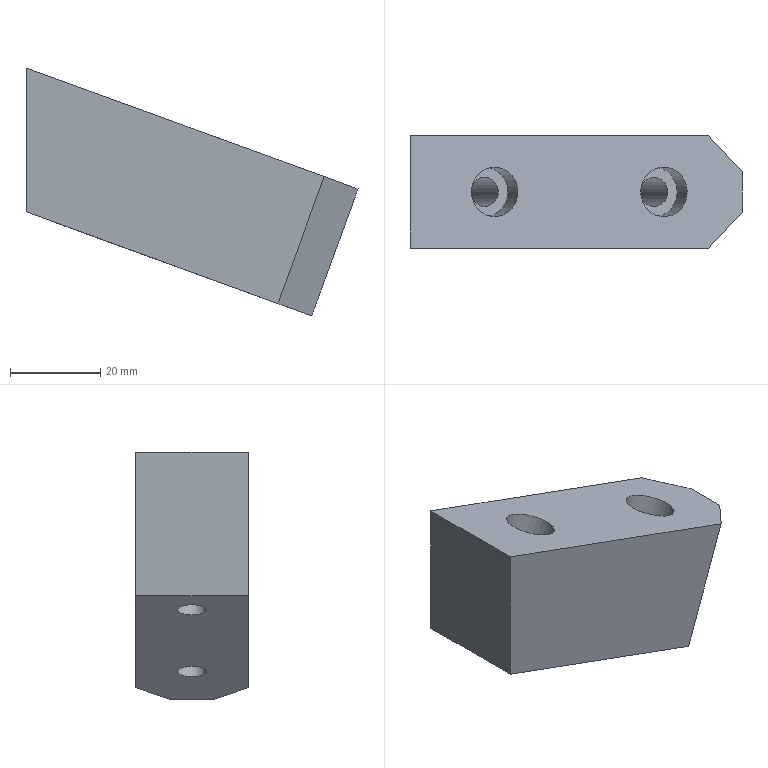Part | STEP file | P011002S002-009 | 1 solid | 14 faces | box 73.728 x 25 x 55.026 mm | volume 50035 mm3 | plane 10 | cylinder 4 | commonest cylinder face diameters 6.5 x2 11 x2
STEP:
#1=CARTESIAN_POINT('',(0.,0.,0.));
#2=DIRECTION('',(0.,0.,1.));
#3=DIRECTION('',(1.,0.,0.));
#4=AXIS2_PLACEMENT_3D('',#1,#2,#3);
#5=CARTESIAN_POINT('',(214.175,15.,-62.861));
#6=VERTEX_POINT('',#5);
#7=CARTESIAN_POINT('',(211.121,15.,-61.749));
#8=DIRECTION('',(-0.342,0.,-0.9397));
#9=DIRECTION('',(0.9397,0.,-0.342));
#10=AXIS2_PLACEMENT_3D('',#7,#8,#9);
#11=CIRCLE('',#10,3.25);
#12=CARTESIAN_POINT('',(219.07,-90.,-64.643));
#13=DIRECTION('',(0.342,0.,0.9397));
#14=DIRECTION('',(-0.9397,0.,0.342));
#15=AXIS2_PLACEMENT_3D('',#12,#13,#14);
#16=PLANE('',#15);
#17=CARTESIAN_POINT('',(5.21,-105.));
#18=CARTESIAN_POINT('',(5.21,-99.371));
#19=CARTESIAN_POINT('',(10.085,-102.185));
#20=CARTESIAN_POINT('',(14.96,-105.));
#21=CARTESIAN_POINT('',(10.085,-107.815));
#22=CARTESIAN_POINT('',(5.21,-110.629));
#23=CARTESIAN_POINT('',(5.21,-105.));
#24=(BOUNDED_CURVE()B_SPLINE_CURVE(2,(#17,#18,#19,#20,#21,#22,#23),.UNSPECIFIED.,.T.,.F.)B_SPLINE_CURVE_WITH_KNOTS((1,2,2,2,2,1),(-2.094,0.,2.094,4.189,6.283,8.378),.UNSPECIFIED.)CURVE()GEOMETRIC_REPRESENTATION_ITEM()RATIONAL_B_SPLINE_CURVE((1.,0.5,1.,0.5,1.,0.5,1.))REPRESENTATION_ITEM(''));
#25=(GEOMETRIC_REPRESENTATION_CONTEXT(2)PARAMETRIC_REPRESENTATION_CONTEXT()REPRESENTATION_CONTEXT('',''));
#26=DEFINITIONAL_REPRESENTATION('',(#24),#25);
#27=PCURVE('',#16,#26);
#28=CARTESIAN_POINT('',(221.382,15.,-33.559));
#29=DIRECTION('',(-0.342,0.,-0.9397));
#30=DIRECTION('',(0.9397,0.,-0.342));
#31=AXIS2_PLACEMENT_3D('',#28,#29,#30);
#32=CYLINDRICAL_SURFACE('',#31,3.25);
#33=CARTESIAN_POINT('',(0.,30.));
#34=DIRECTION('',(1.,0.));
#35=VECTOR('',#34,1.);
#36=LINE('',#33,#35);
#37=(GEOMETRIC_REPRESENTATION_CONTEXT(2)PARAMETRIC_REPRESENTATION_CONTEXT()REPRESENTATION_CONTEXT('',''));
#38=DEFINITIONAL_REPRESENTATION('',(#36),#37);
#39=PCURVE('',#32,#38);
#40=SURFACE_CURVE('',#11,(#27,#39),.PCURVE_S1.);
#41=EDGE_CURVE('',#6,#6,#40,.T.);
#42=ORIENTED_EDGE('',*,*,#41,.F.);
#43=EDGE_LOOP('',(#42));
#44=FACE_BOUND('',#43,.T.);
#45=CARTESIAN_POINT('',(220.95,2.5,-65.327));
#46=VERTEX_POINT('',#45);
#47=CARTESIAN_POINT('',(165.,2.5,-44.963));
#48=VERTEX_POINT('',#47);
#49=CARTESIAN_POINT('',(219.07,2.5,-64.643));
#50=DIRECTION('',(-0.9397,0.,0.342));
#51=VECTOR('',#50,1.);
#52=LINE('',#49,#51);
#53=CARTESIAN_POINT('',(0.,-92.5));
#54=DIRECTION('',(1.,0.));
#55=VECTOR('',#54,1.);
#56=LINE('',#53,#55);
#57=(GEOMETRIC_REPRESENTATION_CONTEXT(2)PARAMETRIC_REPRESENTATION_CONTEXT()REPRESENTATION_CONTEXT('',''));
#58=DEFINITIONAL_REPRESENTATION('',(#56),#57);
#59=PCURVE('',#16,#58);
#60=CARTESIAN_POINT('',(228.899,2.5,-52.257));
#61=DIRECTION('',(0.,-1.,0.));
#62=DIRECTION('',(0.342,0.,0.9397));
#63=AXIS2_PLACEMENT_3D('',#60,#61,#62);
#64=PLANE('',#63);
#65=CARTESIAN_POINT('',(-15.,5.));
#66=DIRECTION('',(0.,1.));
#67=VECTOR('',#66,1.);
#68=LINE('',#65,#67);
#69=(GEOMETRIC_REPRESENTATION_CONTEXT(2)PARAMETRIC_REPRESENTATION_CONTEXT()REPRESENTATION_CONTEXT('',''));
#70=DEFINITIONAL_REPRESENTATION('',(#68),#69);
#71=PCURVE('',#64,#70);
#72=SURFACE_CURVE('',#52,(#59,#71),.PCURVE_S1.);
#73=EDGE_CURVE('',#46,#48,#72,.T.);
#74=ORIENTED_EDGE('',*,*,#73,.T.);
#75=CARTESIAN_POINT('',(165.,27.5,-44.963));
#76=VERTEX_POINT('',#75);
#77=CARTESIAN_POINT('',(165.,-90.,-44.963));
#78=DIRECTION('',(0.,1.,0.));
#79=VECTOR('',#78,1.);
#80=LINE('',#77,#79);
#81=CARTESIAN_POINT('',(57.54,0.));
#82=DIRECTION('',(0.,-1.));
#83=VECTOR('',#82,1.);
#84=LINE('',#81,#83);
#85=(GEOMETRIC_REPRESENTATION_CONTEXT(2)PARAMETRIC_REPRESENTATION_CONTEXT()REPRESENTATION_CONTEXT('',''));
#86=DEFINITIONAL_REPRESENTATION('',(#84),#85);
#87=PCURVE('',#16,#86);
#88=CARTESIAN_POINT('',(165.,-10.,0.));
#89=DIRECTION('',(-1.,0.,0.));
#90=DIRECTION('',(0.,0.,-1.));
#91=AXIS2_PLACEMENT_3D('',#88,#89,#90);
#92=PLANE('',#91);
#93=CARTESIAN_POINT('',(44.963,80.));
#94=DIRECTION('',(0.,-1.));
#95=VECTOR('',#94,1.);
#96=LINE('',#93,#95);
#97=(GEOMETRIC_REPRESENTATION_CONTEXT(2)PARAMETRIC_REPRESENTATION_CONTEXT()REPRESENTATION_CONTEXT('',''));
#98=DEFINITIONAL_REPRESENTATION('',(#96),#97);
#99=PCURVE('',#92,#98);
#100=SURFACE_CURVE('',#80,(#87,#99),.PCURVE_S1.);
#101=EDGE_CURVE('',#48,#76,#100,.T.);
#102=ORIENTED_EDGE('',*,*,#101,.T.);
#103=CARTESIAN_POINT('',(220.95,27.5,-65.327));
#104=VERTEX_POINT('',#103);
#105=CARTESIAN_POINT('',(219.07,27.5,-64.643));
#106=DIRECTION('',(0.9397,0.,-0.342));
#107=VECTOR('',#106,1.);
#108=LINE('',#105,#107);
#109=CARTESIAN_POINT('',(0.,-117.5));
#110=DIRECTION('',(-1.,0.));
#111=VECTOR('',#110,1.);
#112=LINE('',#109,#111);
#113=(GEOMETRIC_REPRESENTATION_CONTEXT(2)PARAMETRIC_REPRESENTATION_CONTEXT()REPRESENTATION_CONTEXT('',''));
#114=DEFINITIONAL_REPRESENTATION('',(#112),#113);
#115=PCURVE('',#16,#114);
#116=CARTESIAN_POINT('',(228.899,27.5,-52.257));
#117=DIRECTION('',(0.,1.,0.));
#118=DIRECTION('',(-0.342,0.,-0.9397));
#119=AXIS2_PLACEMENT_3D('',#116,#117,#118);
#120=PLANE('',#119);
#121=CARTESIAN_POINT('',(15.,5.));
#122=DIRECTION('',(0.,-1.));
#123=VECTOR('',#122,1.);
#124=LINE('',#121,#123);
#125=(GEOMETRIC_REPRESENTATION_CONTEXT(2)PARAMETRIC_REPRESENTATION_CONTEXT()REPRESENTATION_CONTEXT('',''));
#126=DEFINITIONAL_REPRESENTATION('',(#124),#125);
#127=PCURVE('',#120,#126);
#128=SURFACE_CURVE('',#108,(#115,#127),.PCURVE_S1.);
#129=EDGE_CURVE('',#76,#104,#128,.T.);
#130=ORIENTED_EDGE('',*,*,#129,.T.);
#131=CARTESIAN_POINT('',(228.467,19.5,-68.063));
#132=VERTEX_POINT('',#131);
#133=CARTESIAN_POINT('',(228.467,19.5,-68.063));
#134=DIRECTION('',(-0.6645,0.7071,0.2418));
#135=VECTOR('',#134,1.);
#136=LINE('',#133,#135);
#137=CARTESIAN_POINT('',(-10.,-109.5));
#138=DIRECTION('',(0.7071,-0.7071));
#139=VECTOR('',#138,1.);
#140=LINE('',#137,#139);
#141=(GEOMETRIC_REPRESENTATION_CONTEXT(2)PARAMETRIC_REPRESENTATION_CONTEXT()REPRESENTATION_CONTEXT('',''));
#142=DEFINITIONAL_REPRESENTATION('',(#140),#141);
#143=PCURVE('',#16,#142);
#144=CARTESIAN_POINT('',(233.598,19.5,-53.967));
#145=DIRECTION('',(-0.6645,-0.7071,0.2418));
#146=DIRECTION('',(-0.7287,0.6848,0.));
#147=AXIS2_PLACEMENT_3D('',#144,#145,#146);
#148=PLANE('',#147);
#149=CARTESIAN_POINT('',(3.739,14.527));
#150=DIRECTION('',(0.9684,-0.2492));
#151=VECTOR('',#150,1.);
#152=LINE('',#149,#151);
#153=(GEOMETRIC_REPRESENTATION_CONTEXT(2)PARAMETRIC_REPRESENTATION_CONTEXT()REPRESENTATION_CONTEXT('',''));
#154=DEFINITIONAL_REPRESENTATION('',(#152),#153);
#155=PCURVE('',#148,#154);
#156=SURFACE_CURVE('',#136,(#143,#155),.PCURVE_S1.);
#157=EDGE_CURVE('',#132,#104,#156,.T.);
#158=ORIENTED_EDGE('',*,*,#157,.F.);
#159=CARTESIAN_POINT('',(228.467,10.5,-68.063));
#160=VERTEX_POINT('',#159);
#161=CARTESIAN_POINT('',(228.467,-90.,-68.063));
#162=DIRECTION('',(0.,-1.,0.));
#163=VECTOR('',#162,1.);
#164=LINE('',#161,#163);
#165=CARTESIAN_POINT('',(-10.,0.));
#166=DIRECTION('',(0.,1.));
#167=VECTOR('',#166,1.);
#168=LINE('',#165,#167);
#169=(GEOMETRIC_REPRESENTATION_CONTEXT(2)PARAMETRIC_REPRESENTATION_CONTEXT()REPRESENTATION_CONTEXT('',''));
#170=DEFINITIONAL_REPRESENTATION('',(#168),#169);
#171=PCURVE('',#16,#170);
#172=CARTESIAN_POINT('',(233.598,10.,-53.967));
#173=DIRECTION('',(0.9397,0.,-0.342));
#174=DIRECTION('',(0.342,0.,0.9397));
#175=AXIS2_PLACEMENT_3D('',#172,#173,#174);
#176=PLANE('',#175);
#177=CARTESIAN_POINT('',(-15.,100.));
#178=DIRECTION('',(0.,1.));
#179=VECTOR('',#178,1.);
#180=LINE('',#177,#179);
#181=(GEOMETRIC_REPRESENTATION_CONTEXT(2)PARAMETRIC_REPRESENTATION_CONTEXT()REPRESENTATION_CONTEXT('',''));
#182=DEFINITIONAL_REPRESENTATION('',(#180),#181);
#183=PCURVE('',#176,#182);
#184=SURFACE_CURVE('',#164,(#171,#183),.PCURVE_S1.);
#185=EDGE_CURVE('',#132,#160,#184,.T.);
#186=ORIENTED_EDGE('',*,*,#185,.T.);
#187=CARTESIAN_POINT('',(220.95,2.5,-65.327));
#188=DIRECTION('',(0.6645,0.7071,-0.2418));
#189=VECTOR('',#188,1.);
#190=LINE('',#187,#189);
#191=CARTESIAN_POINT('',(-2.,-92.5));
#192=DIRECTION('',(-0.7071,-0.7071));
#193=VECTOR('',#192,1.);
#194=LINE('',#191,#193);
#195=(GEOMETRIC_REPRESENTATION_CONTEXT(2)PARAMETRIC_REPRESENTATION_CONTEXT()REPRESENTATION_CONTEXT('',''));
#196=DEFINITIONAL_REPRESENTATION('',(#194),#195);
#197=PCURVE('',#16,#196);
#198=CARTESIAN_POINT('',(226.08,2.5,-51.231));
#199=DIRECTION('',(-0.6645,0.7071,0.2418));
#200=DIRECTION('',(0.7287,0.6848,0.));
#201=AXIS2_PLACEMENT_3D('',#198,#199,#200);
#202=PLANE('',#201);
#203=CARTESIAN_POINT('',(-3.739,14.527));
#204=DIRECTION('',(0.9684,0.2492));
#205=VECTOR('',#204,1.);
#206=LINE('',#203,#205);
#207=(GEOMETRIC_REPRESENTATION_CONTEXT(2)PARAMETRIC_REPRESENTATION_CONTEXT()REPRESENTATION_CONTEXT('',''));
#208=DEFINITIONAL_REPRESENTATION('',(#206),#207);
#209=PCURVE('',#202,#208);
#210=SURFACE_CURVE('',#190,(#197,#209),.PCURVE_S1.);
#211=EDGE_CURVE('',#46,#160,#210,.T.);
#212=ORIENTED_EDGE('',*,*,#211,.F.);
#213=EDGE_LOOP('',(#74,#102,#130,#158,#186,#212));
#214=FACE_BOUND('',#213,.T.);
#215=CARTESIAN_POINT('',(176.587,15.,-49.18));
#216=VERTEX_POINT('',#215);
#217=CARTESIAN_POINT('',(173.533,15.,-48.069));
#218=DIRECTION('',(-0.342,0.,-0.9397));
#219=DIRECTION('',(0.9397,0.,-0.342));
#220=AXIS2_PLACEMENT_3D('',#217,#218,#219);
#221=CIRCLE('',#220,3.25);
#222=CARTESIAN_POINT('',(45.21,-105.));
#223=CARTESIAN_POINT('',(45.21,-99.371));
#224=CARTESIAN_POINT('',(50.085,-102.185));
#225=CARTESIAN_POINT('',(54.96,-105.));
#226=CARTESIAN_POINT('',(50.085,-107.815));
#227=CARTESIAN_POINT('',(45.21,-110.629));
#228=CARTESIAN_POINT('',(45.21,-105.));
#229=(BOUNDED_CURVE()B_SPLINE_CURVE(2,(#222,#223,#224,#225,#226,#227,#228),.UNSPECIFIED.,.T.,.F.)B_SPLINE_CURVE_WITH_KNOTS((1,2,2,2,2,1),(-2.094,0.,2.094,4.189,6.283,8.378),.UNSPECIFIED.)CURVE()GEOMETRIC_REPRESENTATION_ITEM()RATIONAL_B_SPLINE_CURVE((1.,0.5,1.,0.5,1.,0.5,1.))REPRESENTATION_ITEM(''));
#230=(GEOMETRIC_REPRESENTATION_CONTEXT(2)PARAMETRIC_REPRESENTATION_CONTEXT()REPRESENTATION_CONTEXT('',''));
#231=DEFINITIONAL_REPRESENTATION('',(#229),#230);
#232=PCURVE('',#16,#231);
#233=CARTESIAN_POINT('',(183.794,15.,-19.878));
#234=DIRECTION('',(-0.342,0.,-0.9397));
#235=DIRECTION('',(0.9397,0.,-0.342));
#236=AXIS2_PLACEMENT_3D('',#233,#234,#235);
#237=CYLINDRICAL_SURFACE('',#236,3.25);
#238=CARTESIAN_POINT('',(0.,30.));
#239=DIRECTION('',(1.,0.));
#240=VECTOR('',#239,1.);
#241=LINE('',#238,#240);
#242=(GEOMETRIC_REPRESENTATION_CONTEXT(2)PARAMETRIC_REPRESENTATION_CONTEXT()REPRESENTATION_CONTEXT('',''));
#243=DEFINITIONAL_REPRESENTATION('',(#241),#242);
#244=PCURVE('',#237,#243);
#245=SURFACE_CURVE('',#221,(#232,#244),.PCURVE_S1.);
#246=EDGE_CURVE('',#216,#216,#245,.T.);
#247=ORIENTED_EDGE('',*,*,#246,.F.);
#248=EDGE_LOOP('',(#247));
#249=FACE_BOUND('',#248,.T.);
#250=ADVANCED_FACE('',(#44,#214,#249),#16,.F.);
#251=CARTESIAN_POINT('',(165.,2.5,-13.037));
#252=VERTEX_POINT('',#251);
#253=CARTESIAN_POINT('',(231.21,2.5,-37.136));
#254=VERTEX_POINT('',#253);
#255=CARTESIAN_POINT('',(234.029,2.5,-38.162));
#256=DIRECTION('',(0.9397,0.,-0.342));
#257=VECTOR('',#256,1.);
#258=LINE('',#255,#257);
#259=CARTESIAN_POINT('',(15.,0.));
#260=DIRECTION('',(0.,-1.));
#261=VECTOR('',#260,1.);
#262=LINE('',#259,#261);
#263=(GEOMETRIC_REPRESENTATION_CONTEXT(2)PARAMETRIC_REPRESENTATION_CONTEXT()REPRESENTATION_CONTEXT('',''));
#264=DEFINITIONAL_REPRESENTATION('',(#262),#263);
#265=PCURVE('',#64,#264);
#266=CARTESIAN_POINT('',(234.029,10.,-38.162));
#267=DIRECTION('',(0.342,0.,0.9397));
#268=DIRECTION('',(-0.9397,0.,0.342));
#269=AXIS2_PLACEMENT_3D('',#266,#267,#268);
#270=PLANE('',#269);
#271=CARTESIAN_POINT('',(0.,7.5));
#272=DIRECTION('',(-1.,0.));
#273=VECTOR('',#272,1.);
#274=LINE('',#271,#273);
#275=(GEOMETRIC_REPRESENTATION_CONTEXT(2)PARAMETRIC_REPRESENTATION_CONTEXT()REPRESENTATION_CONTEXT('',''));
#276=DEFINITIONAL_REPRESENTATION('',(#274),#275);
#277=PCURVE('',#270,#276);
#278=SURFACE_CURVE('',#258,(#265,#277),.PCURVE_S1.);
#279=EDGE_CURVE('',#252,#254,#278,.T.);
#280=ORIENTED_EDGE('',*,*,#279,.F.);
#281=CARTESIAN_POINT('',(165.,2.5,0.));
#282=DIRECTION('',(0.,0.,-1.));
#283=VECTOR('',#282,1.);
#284=LINE('',#281,#283);
#285=CARTESIAN_POINT('',(27.251,77.919));
#286=DIRECTION('',(-0.9397,-0.342));
#287=VECTOR('',#286,1.);
#288=LINE('',#285,#287);
#289=(GEOMETRIC_REPRESENTATION_CONTEXT(2)PARAMETRIC_REPRESENTATION_CONTEXT()REPRESENTATION_CONTEXT('',''));
#290=DEFINITIONAL_REPRESENTATION('',(#288),#289);
#291=PCURVE('',#64,#290);
#292=CARTESIAN_POINT('',(0.,-12.5));
#293=DIRECTION('',(1.,0.));
#294=VECTOR('',#293,1.);
#295=LINE('',#292,#294);
#296=(GEOMETRIC_REPRESENTATION_CONTEXT(2)PARAMETRIC_REPRESENTATION_CONTEXT()REPRESENTATION_CONTEXT('',''));
#297=DEFINITIONAL_REPRESENTATION('',(#295),#296);
#298=PCURVE('',#92,#297);
#299=SURFACE_CURVE('',#284,(#291,#298),.PCURVE_S1.);
#300=EDGE_CURVE('',#252,#48,#299,.T.);
#301=ORIENTED_EDGE('',*,*,#300,.T.);
#302=ORIENTED_EDGE('',*,*,#73,.F.);
#303=CARTESIAN_POINT('',(226.08,2.5,-51.231));
#304=DIRECTION('',(-0.342,0.,-0.9397));
#305=VECTOR('',#304,1.);
#306=LINE('',#303,#305);
#307=CARTESIAN_POINT('',(0.,3.));
#308=DIRECTION('',(-1.,0.));
#309=VECTOR('',#308,1.);
#310=LINE('',#307,#309);
#311=(GEOMETRIC_REPRESENTATION_CONTEXT(2)PARAMETRIC_REPRESENTATION_CONTEXT()REPRESENTATION_CONTEXT('',''));
#312=DEFINITIONAL_REPRESENTATION('',(#310),#311);
#313=PCURVE('',#64,#312);
#314=CARTESIAN_POINT('',(0.,0.));
#315=DIRECTION('',(-0.2492,0.9684));
#316=VECTOR('',#315,1.);
#317=LINE('',#314,#316);
#318=(GEOMETRIC_REPRESENTATION_CONTEXT(2)PARAMETRIC_REPRESENTATION_CONTEXT()REPRESENTATION_CONTEXT('',''));
#319=DEFINITIONAL_REPRESENTATION('',(#317),#318);
#320=PCURVE('',#202,#319);
#321=SURFACE_CURVE('',#306,(#313,#320),.PCURVE_S1.);
#322=EDGE_CURVE('',#254,#46,#321,.T.);
#323=ORIENTED_EDGE('',*,*,#322,.F.);
#324=EDGE_LOOP('',(#280,#301,#302,#323));
#325=FACE_BOUND('',#324,.T.);
#326=ADVANCED_FACE('',(#325),#64,.T.);
#327=ORIENTED_EDGE('',*,*,#300,.F.);
#328=CARTESIAN_POINT('',(165.,27.5,-13.037));
#329=VERTEX_POINT('',#328);
#330=CARTESIAN_POINT('',(165.,-10.,-13.037));
#331=DIRECTION('',(0.,-1.,0.));
#332=VECTOR('',#331,1.);
#333=LINE('',#330,#332);
#334=CARTESIAN_POINT('',(13.037,0.));
#335=DIRECTION('',(0.,1.));
#336=VECTOR('',#335,1.);
#337=LINE('',#334,#336);
#338=(GEOMETRIC_REPRESENTATION_CONTEXT(2)PARAMETRIC_REPRESENTATION_CONTEXT()REPRESENTATION_CONTEXT('',''));
#339=DEFINITIONAL_REPRESENTATION('',(#337),#338);
#340=PCURVE('',#92,#339);
#341=CARTESIAN_POINT('',(73.46,20.));
#342=DIRECTION('',(0.,1.));
#343=VECTOR('',#342,1.);
#344=LINE('',#341,#343);
#345=(GEOMETRIC_REPRESENTATION_CONTEXT(2)PARAMETRIC_REPRESENTATION_CONTEXT()REPRESENTATION_CONTEXT('',''));
#346=DEFINITIONAL_REPRESENTATION('',(#344),#345);
#347=PCURVE('',#270,#346);
#348=SURFACE_CURVE('',#333,(#340,#347),.PCURVE_S1.);
#349=EDGE_CURVE('',#329,#252,#348,.T.);
#350=ORIENTED_EDGE('',*,*,#349,.F.);
#351=CARTESIAN_POINT('',(165.,27.5,-52.257));
#352=DIRECTION('',(0.,0.,-1.));
#353=VECTOR('',#352,1.);
#354=LINE('',#351,#353);
#355=CARTESIAN_POINT('',(52.257,-37.5));
#356=DIRECTION('',(1.,0.));
#357=VECTOR('',#356,1.);
#358=LINE('',#355,#357);
#359=(GEOMETRIC_REPRESENTATION_CONTEXT(2)PARAMETRIC_REPRESENTATION_CONTEXT()REPRESENTATION_CONTEXT('',''));
#360=DEFINITIONAL_REPRESENTATION('',(#358),#359);
#361=PCURVE('',#92,#360);
#362=CARTESIAN_POINT('',(21.855,60.046));
#363=DIRECTION('',(0.9397,-0.342));
#364=VECTOR('',#363,1.);
#365=LINE('',#362,#364);
#366=(GEOMETRIC_REPRESENTATION_CONTEXT(2)PARAMETRIC_REPRESENTATION_CONTEXT()REPRESENTATION_CONTEXT('',''));
#367=DEFINITIONAL_REPRESENTATION('',(#365),#366);
#368=PCURVE('',#120,#367);
#369=SURFACE_CURVE('',#354,(#361,#368),.PCURVE_S1.);
#370=EDGE_CURVE('',#329,#76,#369,.T.);
#371=ORIENTED_EDGE('',*,*,#370,.T.);
#372=ORIENTED_EDGE('',*,*,#101,.F.);
#373=EDGE_LOOP('',(#327,#350,#371,#372));
#374=FACE_BOUND('',#373,.T.);
#375=ADVANCED_FACE('',(#374),#92,.T.);
#376=ORIENTED_EDGE('',*,*,#129,.F.);
#377=ORIENTED_EDGE('',*,*,#370,.F.);
#378=CARTESIAN_POINT('',(231.21,27.5,-37.136));
#379=VERTEX_POINT('',#378);
#380=CARTESIAN_POINT('',(234.029,27.5,-38.162));
#381=DIRECTION('',(-0.9397,0.,0.342));
#382=VECTOR('',#381,1.);
#383=LINE('',#380,#382);
#384=CARTESIAN_POINT('',(-15.,0.));
#385=DIRECTION('',(0.,1.));
#386=VECTOR('',#385,1.);
#387=LINE('',#384,#386);
#388=(GEOMETRIC_REPRESENTATION_CONTEXT(2)PARAMETRIC_REPRESENTATION_CONTEXT()REPRESENTATION_CONTEXT('',''));
#389=DEFINITIONAL_REPRESENTATION('',(#387),#388);
#390=PCURVE('',#120,#389);
#391=CARTESIAN_POINT('',(0.,-17.5));
#392=DIRECTION('',(1.,0.));
#393=VECTOR('',#392,1.);
#394=LINE('',#391,#393);
#395=(GEOMETRIC_REPRESENTATION_CONTEXT(2)PARAMETRIC_REPRESENTATION_CONTEXT()REPRESENTATION_CONTEXT('',''));
#396=DEFINITIONAL_REPRESENTATION('',(#394),#395);
#397=PCURVE('',#270,#396);
#398=SURFACE_CURVE('',#383,(#390,#397),.PCURVE_S1.);
#399=EDGE_CURVE('',#379,#329,#398,.T.);
#400=ORIENTED_EDGE('',*,*,#399,.F.);
#401=CARTESIAN_POINT('',(226.08,27.5,-51.231));
#402=DIRECTION('',(0.342,0.,0.9397));
#403=VECTOR('',#402,1.);
#404=LINE('',#401,#403);
#405=CARTESIAN_POINT('',(0.,3.));
#406=DIRECTION('',(-1.,0.));
#407=VECTOR('',#406,1.);
#408=LINE('',#405,#407);
#409=(GEOMETRIC_REPRESENTATION_CONTEXT(2)PARAMETRIC_REPRESENTATION_CONTEXT()REPRESENTATION_CONTEXT('',''));
#410=DEFINITIONAL_REPRESENTATION('',(#408),#409);
#411=PCURVE('',#120,#410);
#412=CARTESIAN_POINT('',(10.957,-2.82));
#413=DIRECTION('',(-0.2492,-0.9684));
#414=VECTOR('',#413,1.);
#415=LINE('',#412,#414);
#416=(GEOMETRIC_REPRESENTATION_CONTEXT(2)PARAMETRIC_REPRESENTATION_CONTEXT()REPRESENTATION_CONTEXT('',''));
#417=DEFINITIONAL_REPRESENTATION('',(#415),#416);
#418=PCURVE('',#148,#417);
#419=SURFACE_CURVE('',#404,(#411,#418),.PCURVE_S1.);
#420=EDGE_CURVE('',#104,#379,#419,.T.);
#421=ORIENTED_EDGE('',*,*,#420,.F.);
#422=EDGE_LOOP('',(#376,#377,#400,#421));
#423=FACE_BOUND('',#422,.T.);
#424=ADVANCED_FACE('',(#423),#120,.T.);
#425=CARTESIAN_POINT('',(216.213,15.,-31.677));
#426=VERTEX_POINT('',#425);
#427=CARTESIAN_POINT('',(221.382,15.,-33.559));
#428=DIRECTION('',(-0.342,0.,-0.9397));
#429=DIRECTION('',(-0.9397,0.,0.342));
#430=AXIS2_PLACEMENT_3D('',#427,#428,#429);
#431=CIRCLE('',#430,5.5);
#432=CARTESIAN_POINT('',(18.96,-5.));
#433=CARTESIAN_POINT('',(18.96,-14.526));
#434=CARTESIAN_POINT('',(10.71,-9.763));
#435=CARTESIAN_POINT('',(2.46,-5.));
#436=CARTESIAN_POINT('',(10.71,-0.2369));
#437=CARTESIAN_POINT('',(18.96,4.526));
#438=CARTESIAN_POINT('',(18.96,-5.));
#439=(BOUNDED_CURVE()B_SPLINE_CURVE(2,(#432,#433,#434,#435,#436,#437,#438),.UNSPECIFIED.,.T.,.F.)B_SPLINE_CURVE_WITH_KNOTS((1,2,2,2,2,1),(-2.094,0.,2.094,4.189,6.283,8.378),.UNSPECIFIED.)CURVE()GEOMETRIC_REPRESENTATION_ITEM()RATIONAL_B_SPLINE_CURVE((1.,0.5,1.,0.5,1.,0.5,1.))REPRESENTATION_ITEM(''));
#440=(GEOMETRIC_REPRESENTATION_CONTEXT(2)PARAMETRIC_REPRESENTATION_CONTEXT()REPRESENTATION_CONTEXT('',''));
#441=DEFINITIONAL_REPRESENTATION('',(#439),#440);
#442=PCURVE('',#270,#441);
#443=CARTESIAN_POINT('',(221.382,15.,-33.559));
#444=DIRECTION('',(-0.342,0.,-0.9397));
#445=DIRECTION('',(0.9397,0.,-0.342));
#446=AXIS2_PLACEMENT_3D('',#443,#444,#445);
#447=CYLINDRICAL_SURFACE('',#446,5.5);
#448=CARTESIAN_POINT('',(3.142,0.));
#449=DIRECTION('',(1.,0.));
#450=VECTOR('',#449,1.);
#451=LINE('',#448,#450);
#452=(GEOMETRIC_REPRESENTATION_CONTEXT(2)PARAMETRIC_REPRESENTATION_CONTEXT()REPRESENTATION_CONTEXT('',''));
#453=DEFINITIONAL_REPRESENTATION('',(#451),#452);
#454=PCURVE('',#447,#453);
#455=SURFACE_CURVE('',#431,(#442,#454),.PCURVE_S1.);
#456=EDGE_CURVE('',#426,#426,#455,.T.);
#457=ORIENTED_EDGE('',*,*,#456,.T.);
#458=EDGE_LOOP('',(#457));
#459=FACE_BOUND('',#458,.T.);
#460=CARTESIAN_POINT('',(178.626,15.,-17.997));
#461=VERTEX_POINT('',#460);
#462=CARTESIAN_POINT('',(183.794,15.,-19.878));
#463=DIRECTION('',(-0.342,0.,-0.9397));
#464=DIRECTION('',(-0.9397,0.,0.342));
#465=AXIS2_PLACEMENT_3D('',#462,#463,#464);
#466=CIRCLE('',#465,5.5);
#467=CARTESIAN_POINT('',(58.96,-5.));
#468=CARTESIAN_POINT('',(58.96,-14.526));
#469=CARTESIAN_POINT('',(50.71,-9.763));
#470=CARTESIAN_POINT('',(42.46,-5.));
#471=CARTESIAN_POINT('',(50.71,-0.2369));
#472=CARTESIAN_POINT('',(58.96,4.526));
#473=CARTESIAN_POINT('',(58.96,-5.));
#474=(BOUNDED_CURVE()B_SPLINE_CURVE(2,(#467,#468,#469,#470,#471,#472,#473),.UNSPECIFIED.,.T.,.F.)B_SPLINE_CURVE_WITH_KNOTS((1,2,2,2,2,1),(-2.094,0.,2.094,4.189,6.283,8.378),.UNSPECIFIED.)CURVE()GEOMETRIC_REPRESENTATION_ITEM()RATIONAL_B_SPLINE_CURVE((1.,0.5,1.,0.5,1.,0.5,1.))REPRESENTATION_ITEM(''));
#475=(GEOMETRIC_REPRESENTATION_CONTEXT(2)PARAMETRIC_REPRESENTATION_CONTEXT()REPRESENTATION_CONTEXT('',''));
#476=DEFINITIONAL_REPRESENTATION('',(#474),#475);
#477=PCURVE('',#270,#476);
#478=CARTESIAN_POINT('',(183.794,15.,-19.878));
#479=DIRECTION('',(-0.342,0.,-0.9397));
#480=DIRECTION('',(0.9397,0.,-0.342));
#481=AXIS2_PLACEMENT_3D('',#478,#479,#480);
#482=CYLINDRICAL_SURFACE('',#481,5.5);
#483=CARTESIAN_POINT('',(3.142,0.));
#484=DIRECTION('',(1.,0.));
#485=VECTOR('',#484,1.);
#486=LINE('',#483,#485);
#487=(GEOMETRIC_REPRESENTATION_CONTEXT(2)PARAMETRIC_REPRESENTATION_CONTEXT()REPRESENTATION_CONTEXT('',''));
#488=DEFINITIONAL_REPRESENTATION('',(#486),#487);
#489=PCURVE('',#482,#488);
#490=SURFACE_CURVE('',#466,(#477,#489),.PCURVE_S1.);
#491=EDGE_CURVE('',#461,#461,#490,.T.);
#492=ORIENTED_EDGE('',*,*,#491,.T.);
#493=EDGE_LOOP('',(#492));
#494=FACE_BOUND('',#493,.T.);
#495=CARTESIAN_POINT('',(238.728,10.5,-39.872));
#496=VERTEX_POINT('',#495);
#497=CARTESIAN_POINT('',(238.728,19.5,-39.872));
#498=VERTEX_POINT('',#497);
#499=CARTESIAN_POINT('',(238.728,10.,-39.872));
#500=DIRECTION('',(0.,1.,0.));
#501=VECTOR('',#500,1.);
#502=LINE('',#499,#501);
#503=CARTESIAN_POINT('',(-5.,0.));
#504=DIRECTION('',(0.,-1.));
#505=VECTOR('',#504,1.);
#506=LINE('',#503,#505);
#507=(GEOMETRIC_REPRESENTATION_CONTEXT(2)PARAMETRIC_REPRESENTATION_CONTEXT()REPRESENTATION_CONTEXT('',''));
#508=DEFINITIONAL_REPRESENTATION('',(#506),#507);
#509=PCURVE('',#270,#508);
#510=CARTESIAN_POINT('',(15.,0.));
#511=DIRECTION('',(0.,-1.));
#512=VECTOR('',#511,1.);
#513=LINE('',#510,#512);
#514=(GEOMETRIC_REPRESENTATION_CONTEXT(2)PARAMETRIC_REPRESENTATION_CONTEXT()REPRESENTATION_CONTEXT('',''));
#515=DEFINITIONAL_REPRESENTATION('',(#513),#514);
#516=PCURVE('',#176,#515);
#517=SURFACE_CURVE('',#502,(#509,#516),.PCURVE_S1.);
#518=EDGE_CURVE('',#496,#498,#517,.T.);
#519=ORIENTED_EDGE('',*,*,#518,.T.);
#520=CARTESIAN_POINT('',(240.842,17.25,-40.642));
#521=DIRECTION('',(0.6645,-0.7071,-0.2418));
#522=VECTOR('',#521,1.);
#523=LINE('',#520,#522);
#524=CARTESIAN_POINT('',(-7.25,-7.25));
#525=DIRECTION('',(-0.7071,0.7071));
#526=VECTOR('',#525,1.);
#527=LINE('',#524,#526);
#528=(GEOMETRIC_REPRESENTATION_CONTEXT(2)PARAMETRIC_REPRESENTATION_CONTEXT()REPRESENTATION_CONTEXT('',''));
#529=DEFINITIONAL_REPRESENTATION('',(#527),#528);
#530=PCURVE('',#270,#529);
#531=CARTESIAN_POINT('',(-6.82,-13.734));
#532=DIRECTION('',(-0.9684,0.2492));
#533=VECTOR('',#532,1.);
#534=LINE('',#531,#533);
#535=(GEOMETRIC_REPRESENTATION_CONTEXT(2)PARAMETRIC_REPRESENTATION_CONTEXT()REPRESENTATION_CONTEXT('',''));
#536=DEFINITIONAL_REPRESENTATION('',(#534),#535);
#537=PCURVE('',#148,#536);
#538=SURFACE_CURVE('',#523,(#530,#537),.PCURVE_S1.);
#539=EDGE_CURVE('',#379,#498,#538,.T.);
#540=ORIENTED_EDGE('',*,*,#539,.F.);
#541=ORIENTED_EDGE('',*,*,#399,.T.);
#542=ORIENTED_EDGE('',*,*,#349,.T.);
#543=ORIENTED_EDGE('',*,*,#279,.T.);
#544=CARTESIAN_POINT('',(236.144,7.75,-38.932));
#545=DIRECTION('',(-0.6645,-0.7071,0.2418));
#546=VECTOR('',#545,1.);
#547=LINE('',#544,#546);
#548=CARTESIAN_POINT('',(-2.25,2.25));
#549=DIRECTION('',(0.7071,0.7071));
#550=VECTOR('',#549,1.);
#551=LINE('',#548,#550);
#552=(GEOMETRIC_REPRESENTATION_CONTEXT(2)PARAMETRIC_REPRESENTATION_CONTEXT()REPRESENTATION_CONTEXT('',''));
#553=DEFINITIONAL_REPRESENTATION('',(#551),#552);
#554=PCURVE('',#270,#553);
#555=CARTESIAN_POINT('',(10.929,-12.676));
#556=DIRECTION('',(-0.9684,-0.2492));
#557=VECTOR('',#556,1.);
#558=LINE('',#555,#557);
#559=(GEOMETRIC_REPRESENTATION_CONTEXT(2)PARAMETRIC_REPRESENTATION_CONTEXT()REPRESENTATION_CONTEXT('',''));
#560=DEFINITIONAL_REPRESENTATION('',(#558),#559);
#561=PCURVE('',#202,#560);
#562=SURFACE_CURVE('',#547,(#554,#561),.PCURVE_S1.);
#563=EDGE_CURVE('',#496,#254,#562,.T.);
#564=ORIENTED_EDGE('',*,*,#563,.F.);
#565=EDGE_LOOP('',(#519,#540,#541,#542,#543,#564));
#566=FACE_BOUND('',#565,.T.);
#567=ADVANCED_FACE('',(#459,#494,#566),#270,.T.);
#568=ORIENTED_EDGE('',*,*,#185,.F.);
#569=CARTESIAN_POINT('',(233.598,19.5,-53.967));
#570=DIRECTION('',(-0.342,0.,-0.9397));
#571=VECTOR('',#570,1.);
#572=LINE('',#569,#571);
#573=CARTESIAN_POINT('',(0.,-9.5));
#574=DIRECTION('',(-1.,0.));
#575=VECTOR('',#574,1.);
#576=LINE('',#573,#575);
#577=(GEOMETRIC_REPRESENTATION_CONTEXT(2)PARAMETRIC_REPRESENTATION_CONTEXT()REPRESENTATION_CONTEXT('',''));
#578=DEFINITIONAL_REPRESENTATION('',(#576),#577);
#579=PCURVE('',#176,#578);
#580=CARTESIAN_POINT('',(0.,0.));
#581=DIRECTION('',(0.2492,0.9684));
#582=VECTOR('',#581,1.);
#583=LINE('',#580,#582);
#584=(GEOMETRIC_REPRESENTATION_CONTEXT(2)PARAMETRIC_REPRESENTATION_CONTEXT()REPRESENTATION_CONTEXT('',''));
#585=DEFINITIONAL_REPRESENTATION('',(#583),#584);
#586=PCURVE('',#148,#585);
#587=SURFACE_CURVE('',#572,(#579,#586),.PCURVE_S1.);
#588=EDGE_CURVE('',#498,#132,#587,.T.);
#589=ORIENTED_EDGE('',*,*,#588,.F.);
#590=ORIENTED_EDGE('',*,*,#518,.F.);
#591=CARTESIAN_POINT('',(233.598,10.5,-53.967));
#592=DIRECTION('',(0.342,0.,0.9397));
#593=VECTOR('',#592,1.);
#594=LINE('',#591,#593);
#595=CARTESIAN_POINT('',(0.,-0.5));
#596=DIRECTION('',(1.,0.));
#597=VECTOR('',#596,1.);
#598=LINE('',#595,#597);
#599=(GEOMETRIC_REPRESENTATION_CONTEXT(2)PARAMETRIC_REPRESENTATION_CONTEXT()REPRESENTATION_CONTEXT('',''));
#600=DEFINITIONAL_REPRESENTATION('',(#598),#599);
#601=PCURVE('',#176,#600);
#602=CARTESIAN_POINT('',(10.957,2.82));
#603=DIRECTION('',(0.2492,-0.9684));
#604=VECTOR('',#603,1.);
#605=LINE('',#602,#604);
#606=(GEOMETRIC_REPRESENTATION_CONTEXT(2)PARAMETRIC_REPRESENTATION_CONTEXT()REPRESENTATION_CONTEXT('',''));
#607=DEFINITIONAL_REPRESENTATION('',(#605),#606);
#608=PCURVE('',#202,#607);
#609=SURFACE_CURVE('',#594,(#601,#608),.PCURVE_S1.);
#610=EDGE_CURVE('',#160,#496,#609,.T.);
#611=ORIENTED_EDGE('',*,*,#610,.F.);
#612=EDGE_LOOP('',(#568,#589,#590,#611));
#613=FACE_BOUND('',#612,.T.);
#614=ADVANCED_FACE('',(#613),#176,.T.);
#615=ORIENTED_EDGE('',*,*,#539,.T.);
#616=ORIENTED_EDGE('',*,*,#588,.T.);
#617=ORIENTED_EDGE('',*,*,#157,.T.);
#618=ORIENTED_EDGE('',*,*,#420,.T.);
#619=EDGE_LOOP('',(#615,#616,#617,#618));
#620=FACE_BOUND('',#619,.T.);
#621=ADVANCED_FACE('',(#620),#148,.F.);
#622=ORIENTED_EDGE('',*,*,#563,.T.);
#623=ORIENTED_EDGE('',*,*,#322,.T.);
#624=ORIENTED_EDGE('',*,*,#211,.T.);
#625=ORIENTED_EDGE('',*,*,#610,.T.);
#626=EDGE_LOOP('',(#622,#623,#624,#625));
#627=FACE_BOUND('',#626,.T.);
#628=ADVANCED_FACE('',(#627),#202,.F.);
#629=ORIENTED_EDGE('',*,*,#246,.F.);
#630=CARTESIAN_POINT('',(184.625,15.,-27.097));
#631=VERTEX_POINT('',#630);
#632=CARTESIAN_POINT('',(184.625,15.,-27.097));
#633=CARTESIAN_POINT('',(176.587,15.,-49.18));
#634=B_SPLINE_CURVE_WITH_KNOTS('',1,(#632,#633),.UNSPECIFIED.,.F.,.F.,(2,2),(6.5,30.),.PIECEWISE_BEZIER_KNOTS.);
#635=CARTESIAN_POINT('',(0.,0.));
#636=DIRECTION('',(0.,1.));
#637=VECTOR('',#636,1.);
#638=LINE('',#635,#637);
#639=(GEOMETRIC_REPRESENTATION_CONTEXT(2)PARAMETRIC_REPRESENTATION_CONTEXT()REPRESENTATION_CONTEXT('',''));
#640=DEFINITIONAL_REPRESENTATION('',(#638),#639);
#641=PCURVE('',#237,#640);
#642=CARTESIAN_POINT('',(6.283,0.));
#643=DIRECTION('',(0.,1.));
#644=VECTOR('',#643,1.);
#645=LINE('',#642,#644);
#646=(GEOMETRIC_REPRESENTATION_CONTEXT(2)PARAMETRIC_REPRESENTATION_CONTEXT()REPRESENTATION_CONTEXT('',''));
#647=DEFINITIONAL_REPRESENTATION('',(#645),#646);
#648=PCURVE('',#237,#647);
#649=SEAM_CURVE('',#634,(#641,#648),.PCURVE_S1.);
#650=EDGE_CURVE('',#631,#216,#649,.T.);
#651=ORIENTED_EDGE('',*,*,#650,.F.);
#652=CARTESIAN_POINT('',(178.517,15.,-24.874));
#653=VERTEX_POINT('',#652);
#654=CARTESIAN_POINT('',(181.571,15.,-25.986));
#655=DIRECTION('',(-0.342,0.,-0.9397));
#656=DIRECTION('',(-0.9397,0.,0.342));
#657=AXIS2_PLACEMENT_3D('',#654,#655,#656);
#658=CIRCLE('',#657,3.25);
#659=CARTESIAN_POINT('',(-3.142,6.5));
#660=DIRECTION('',(1.,0.));
#661=VECTOR('',#660,1.);
#662=LINE('',#659,#661);
#663=(GEOMETRIC_REPRESENTATION_CONTEXT(2)PARAMETRIC_REPRESENTATION_CONTEXT()REPRESENTATION_CONTEXT('',''));
#664=DEFINITIONAL_REPRESENTATION('',(#662),#663);
#665=PCURVE('',#237,#664);
#666=CARTESIAN_POINT('',(199.641,15.,-32.563));
#667=DIRECTION('',(0.342,0.,0.9397));
#668=DIRECTION('',(-0.9397,0.,0.342));
#669=AXIS2_PLACEMENT_3D('',#666,#667,#668);
#670=PLANE('',#669);
#671=CARTESIAN_POINT('',(22.48,0.));
#672=CARTESIAN_POINT('',(22.48,-5.629));
#673=CARTESIAN_POINT('',(17.605,-2.815));
#674=CARTESIAN_POINT('',(12.73,0.));
#675=CARTESIAN_POINT('',(17.605,2.815));
#676=CARTESIAN_POINT('',(22.48,5.629));
#677=CARTESIAN_POINT('',(22.48,0.));
#678=(BOUNDED_CURVE()B_SPLINE_CURVE(2,(#671,#672,#673,#674,#675,#676,#677),.UNSPECIFIED.,.T.,.F.)B_SPLINE_CURVE_WITH_KNOTS((1,2,2,2,2,1),(-2.094,0.,2.094,4.189,6.283,8.378),.UNSPECIFIED.)CURVE()GEOMETRIC_REPRESENTATION_ITEM()RATIONAL_B_SPLINE_CURVE((1.,0.5,1.,0.5,1.,0.5,1.))REPRESENTATION_ITEM(''));
#679=(GEOMETRIC_REPRESENTATION_CONTEXT(2)PARAMETRIC_REPRESENTATION_CONTEXT()REPRESENTATION_CONTEXT('',''));
#680=DEFINITIONAL_REPRESENTATION('',(#678),#679);
#681=PCURVE('',#670,#680);
#682=SURFACE_CURVE('',#658,(#665,#681),.PCURVE_S1.);
#683=EDGE_CURVE('',#631,#653,#682,.T.);
#684=ORIENTED_EDGE('',*,*,#683,.T.);
#685=CARTESIAN_POINT('',(181.571,15.,-25.986));
#686=DIRECTION('',(-0.342,0.,-0.9397));
#687=DIRECTION('',(-0.9397,0.,0.342));
#688=AXIS2_PLACEMENT_3D('',#685,#686,#687);
#689=CIRCLE('',#688,3.25);
#690=CARTESIAN_POINT('',(3.142,6.5));
#691=DIRECTION('',(1.,0.));
#692=VECTOR('',#691,1.);
#693=LINE('',#690,#692);
#694=(GEOMETRIC_REPRESENTATION_CONTEXT(2)PARAMETRIC_REPRESENTATION_CONTEXT()REPRESENTATION_CONTEXT('',''));
#695=DEFINITIONAL_REPRESENTATION('',(#693),#694);
#696=PCURVE('',#237,#695);
#697=CARTESIAN_POINT('',(22.48,0.));
#698=CARTESIAN_POINT('',(22.48,-5.629));
#699=CARTESIAN_POINT('',(17.605,-2.815));
#700=CARTESIAN_POINT('',(12.73,0.));
#701=CARTESIAN_POINT('',(17.605,2.815));
#702=CARTESIAN_POINT('',(22.48,5.629));
#703=CARTESIAN_POINT('',(22.48,0.));
#704=(BOUNDED_CURVE()B_SPLINE_CURVE(2,(#697,#698,#699,#700,#701,#702,#703),.UNSPECIFIED.,.T.,.F.)B_SPLINE_CURVE_WITH_KNOTS((1,2,2,2,2,1),(-2.094,0.,2.094,4.189,6.283,8.378),.UNSPECIFIED.)CURVE()GEOMETRIC_REPRESENTATION_ITEM()RATIONAL_B_SPLINE_CURVE((1.,0.5,1.,0.5,1.,0.5,1.))REPRESENTATION_ITEM(''));
#705=(GEOMETRIC_REPRESENTATION_CONTEXT(2)PARAMETRIC_REPRESENTATION_CONTEXT()REPRESENTATION_CONTEXT('',''));
#706=DEFINITIONAL_REPRESENTATION('',(#704),#705);
#707=PCURVE('',#670,#706);
#708=SURFACE_CURVE('',#689,(#696,#707),.PCURVE_S1.);
#709=EDGE_CURVE('',#653,#631,#708,.T.);
#710=ORIENTED_EDGE('',*,*,#709,.T.);
#711=ORIENTED_EDGE('',*,*,#650,.T.);
#712=EDGE_LOOP('',(#629,#651,#684,#710,#711));
#713=FACE_BOUND('',#712,.F.);
#714=ADVANCED_FACE('',(#713),#237,.F.);
#715=CARTESIAN_POINT('',(176.402,15.,-24.105));
#716=VERTEX_POINT('',#715);
#717=CARTESIAN_POINT('',(181.571,15.,-25.986));
#718=DIRECTION('',(-0.342,0.,-0.9397));
#719=DIRECTION('',(-0.9397,0.,0.342));
#720=AXIS2_PLACEMENT_3D('',#717,#718,#719);
#721=CIRCLE('',#720,5.5);
#722=CARTESIAN_POINT('',(24.73,0.));
#723=CARTESIAN_POINT('',(24.73,-9.526));
#724=CARTESIAN_POINT('',(16.48,-4.763));
#725=CARTESIAN_POINT('',(8.23,0.));
#726=CARTESIAN_POINT('',(16.48,4.763));
#727=CARTESIAN_POINT('',(24.73,9.526));
#728=CARTESIAN_POINT('',(24.73,0.));
#729=(BOUNDED_CURVE()B_SPLINE_CURVE(2,(#722,#723,#724,#725,#726,#727,#728),.UNSPECIFIED.,.T.,.F.)B_SPLINE_CURVE_WITH_KNOTS((1,2,2,2,2,1),(-2.094,0.,2.094,4.189,6.283,8.378),.UNSPECIFIED.)CURVE()GEOMETRIC_REPRESENTATION_ITEM()RATIONAL_B_SPLINE_CURVE((1.,0.5,1.,0.5,1.,0.5,1.))REPRESENTATION_ITEM(''));
#730=(GEOMETRIC_REPRESENTATION_CONTEXT(2)PARAMETRIC_REPRESENTATION_CONTEXT()REPRESENTATION_CONTEXT('',''));
#731=DEFINITIONAL_REPRESENTATION('',(#729),#730);
#732=PCURVE('',#670,#731);
#733=CARTESIAN_POINT('',(3.142,6.5));
#734=DIRECTION('',(1.,0.));
#735=VECTOR('',#734,1.);
#736=LINE('',#733,#735);
#737=(GEOMETRIC_REPRESENTATION_CONTEXT(2)PARAMETRIC_REPRESENTATION_CONTEXT()REPRESENTATION_CONTEXT('',''));
#738=DEFINITIONAL_REPRESENTATION('',(#736),#737);
#739=PCURVE('',#482,#738);
#740=SURFACE_CURVE('',#721,(#732,#739),.PCURVE_S1.);
#741=EDGE_CURVE('',#716,#716,#740,.T.);
#742=ORIENTED_EDGE('',*,*,#741,.F.);
#743=EDGE_LOOP('',(#742));
#744=FACE_BOUND('',#743,.T.);
#745=ORIENTED_EDGE('',*,*,#709,.T.);
#746=ORIENTED_EDGE('',*,*,#683,.T.);
#747=EDGE_LOOP('',(#745,#746));
#748=FACE_BOUND('',#747,.T.);
#749=ADVANCED_FACE('',(#744,#748),#670,.T.);
#750=ORIENTED_EDGE('',*,*,#741,.F.);
#751=CARTESIAN_POINT('',(178.626,15.,-17.997));
#752=CARTESIAN_POINT('',(176.402,15.,-24.105));
#753=B_SPLINE_CURVE_WITH_KNOTS('',1,(#751,#752),.UNSPECIFIED.,.F.,.F.,(2,2),(0.,6.5),.PIECEWISE_BEZIER_KNOTS.);
#754=CARTESIAN_POINT('',(3.142,0.));
#755=DIRECTION('',(0.,1.));
#756=VECTOR('',#755,1.);
#757=LINE('',#754,#756);
#758=(GEOMETRIC_REPRESENTATION_CONTEXT(2)PARAMETRIC_REPRESENTATION_CONTEXT()REPRESENTATION_CONTEXT('',''));
#759=DEFINITIONAL_REPRESENTATION('',(#757),#758);
#760=PCURVE('',#482,#759);
#761=CARTESIAN_POINT('',(9.425,0.));
#762=DIRECTION('',(0.,1.));
#763=VECTOR('',#762,1.);
#764=LINE('',#761,#763);
#765=(GEOMETRIC_REPRESENTATION_CONTEXT(2)PARAMETRIC_REPRESENTATION_CONTEXT()REPRESENTATION_CONTEXT('',''));
#766=DEFINITIONAL_REPRESENTATION('',(#764),#765);
#767=PCURVE('',#482,#766);
#768=SEAM_CURVE('',#753,(#760,#767),.PCURVE_S1.);
#769=EDGE_CURVE('',#461,#716,#768,.T.);
#770=ORIENTED_EDGE('',*,*,#769,.F.);
#771=ORIENTED_EDGE('',*,*,#491,.T.);
#772=ORIENTED_EDGE('',*,*,#769,.T.);
#773=EDGE_LOOP('',(#750,#770,#771,#772));
#774=FACE_BOUND('',#773,.F.);
#775=ADVANCED_FACE('',(#774),#482,.F.);
#776=ORIENTED_EDGE('',*,*,#41,.F.);
#777=CARTESIAN_POINT('',(222.212,15.,-40.778));
#778=VERTEX_POINT('',#777);
#779=CARTESIAN_POINT('',(222.212,15.,-40.778));
#780=CARTESIAN_POINT('',(214.175,15.,-62.861));
#781=B_SPLINE_CURVE_WITH_KNOTS('',1,(#779,#780),.UNSPECIFIED.,.F.,.F.,(2,2),(6.5,30.),.PIECEWISE_BEZIER_KNOTS.);
#782=CARTESIAN_POINT('',(0.,0.));
#783=DIRECTION('',(0.,1.));
#784=VECTOR('',#783,1.);
#785=LINE('',#782,#784);
#786=(GEOMETRIC_REPRESENTATION_CONTEXT(2)PARAMETRIC_REPRESENTATION_CONTEXT()REPRESENTATION_CONTEXT('',''));
#787=DEFINITIONAL_REPRESENTATION('',(#785),#786);
#788=PCURVE('',#32,#787);
#789=CARTESIAN_POINT('',(6.283,0.));
#790=DIRECTION('',(0.,1.));
#791=VECTOR('',#790,1.);
#792=LINE('',#789,#791);
#793=(GEOMETRIC_REPRESENTATION_CONTEXT(2)PARAMETRIC_REPRESENTATION_CONTEXT()REPRESENTATION_CONTEXT('',''));
#794=DEFINITIONAL_REPRESENTATION('',(#792),#793);
#795=PCURVE('',#32,#794);
#796=SEAM_CURVE('',#781,(#788,#795),.PCURVE_S1.);
#797=EDGE_CURVE('',#778,#6,#796,.T.);
#798=ORIENTED_EDGE('',*,*,#797,.F.);
#799=CARTESIAN_POINT('',(216.104,15.,-38.555));
#800=VERTEX_POINT('',#799);
#801=CARTESIAN_POINT('',(219.158,15.,-39.667));
#802=DIRECTION('',(-0.342,0.,-0.9397));
#803=DIRECTION('',(-0.9397,0.,0.342));
#804=AXIS2_PLACEMENT_3D('',#801,#802,#803);
#805=CIRCLE('',#804,3.25);
#806=CARTESIAN_POINT('',(-3.142,6.5));
#807=DIRECTION('',(1.,0.));
#808=VECTOR('',#807,1.);
#809=LINE('',#806,#808);
#810=(GEOMETRIC_REPRESENTATION_CONTEXT(2)PARAMETRIC_REPRESENTATION_CONTEXT()REPRESENTATION_CONTEXT('',''));
#811=DEFINITIONAL_REPRESENTATION('',(#809),#810);
#812=PCURVE('',#32,#811);
#813=CARTESIAN_POINT('',(199.641,15.,-32.563));
#814=DIRECTION('',(0.342,0.,0.9397));
#815=DIRECTION('',(-0.9397,0.,0.342));
#816=AXIS2_PLACEMENT_3D('',#813,#814,#815);
#817=PLANE('',#816);
#818=CARTESIAN_POINT('',(-17.52,0.));
#819=CARTESIAN_POINT('',(-17.52,-5.629));
#820=CARTESIAN_POINT('',(-22.395,-2.815));
#821=CARTESIAN_POINT('',(-27.27,0.));
#822=CARTESIAN_POINT('',(-22.395,2.815));
#823=CARTESIAN_POINT('',(-17.52,5.629));
#824=CARTESIAN_POINT('',(-17.52,0.));
#825=(BOUNDED_CURVE()B_SPLINE_CURVE(2,(#818,#819,#820,#821,#822,#823,#824),.UNSPECIFIED.,.T.,.F.)B_SPLINE_CURVE_WITH_KNOTS((1,2,2,2,2,1),(-2.094,0.,2.094,4.189,6.283,8.378),.UNSPECIFIED.)CURVE()GEOMETRIC_REPRESENTATION_ITEM()RATIONAL_B_SPLINE_CURVE((1.,0.5,1.,0.5,1.,0.5,1.))REPRESENTATION_ITEM(''));
#826=(GEOMETRIC_REPRESENTATION_CONTEXT(2)PARAMETRIC_REPRESENTATION_CONTEXT()REPRESENTATION_CONTEXT('',''));
#827=DEFINITIONAL_REPRESENTATION('',(#825),#826);
#828=PCURVE('',#817,#827);
#829=SURFACE_CURVE('',#805,(#812,#828),.PCURVE_S1.);
#830=EDGE_CURVE('',#778,#800,#829,.T.);
#831=ORIENTED_EDGE('',*,*,#830,.T.);
#832=CARTESIAN_POINT('',(219.158,15.,-39.667));
#833=DIRECTION('',(-0.342,0.,-0.9397));
#834=DIRECTION('',(-0.9397,0.,0.342));
#835=AXIS2_PLACEMENT_3D('',#832,#833,#834);
#836=CIRCLE('',#835,3.25);
#837=CARTESIAN_POINT('',(3.142,6.5));
#838=DIRECTION('',(1.,0.));
#839=VECTOR('',#838,1.);
#840=LINE('',#837,#839);
#841=(GEOMETRIC_REPRESENTATION_CONTEXT(2)PARAMETRIC_REPRESENTATION_CONTEXT()REPRESENTATION_CONTEXT('',''));
#842=DEFINITIONAL_REPRESENTATION('',(#840),#841);
#843=PCURVE('',#32,#842);
#844=CARTESIAN_POINT('',(-17.52,0.));
#845=CARTESIAN_POINT('',(-17.52,-5.629));
#846=CARTESIAN_POINT('',(-22.395,-2.815));
#847=CARTESIAN_POINT('',(-27.27,0.));
#848=CARTESIAN_POINT('',(-22.395,2.815));
#849=CARTESIAN_POINT('',(-17.52,5.629));
#850=CARTESIAN_POINT('',(-17.52,0.));
#851=(BOUNDED_CURVE()B_SPLINE_CURVE(2,(#844,#845,#846,#847,#848,#849,#850),.UNSPECIFIED.,.T.,.F.)B_SPLINE_CURVE_WITH_KNOTS((1,2,2,2,2,1),(-2.094,0.,2.094,4.189,6.283,8.378),.UNSPECIFIED.)CURVE()GEOMETRIC_REPRESENTATION_ITEM()RATIONAL_B_SPLINE_CURVE((1.,0.5,1.,0.5,1.,0.5,1.))REPRESENTATION_ITEM(''));
#852=(GEOMETRIC_REPRESENTATION_CONTEXT(2)PARAMETRIC_REPRESENTATION_CONTEXT()REPRESENTATION_CONTEXT('',''));
#853=DEFINITIONAL_REPRESENTATION('',(#851),#852);
#854=PCURVE('',#817,#853);
#855=SURFACE_CURVE('',#836,(#843,#854),.PCURVE_S1.);
#856=EDGE_CURVE('',#800,#778,#855,.T.);
#857=ORIENTED_EDGE('',*,*,#856,.T.);
#858=ORIENTED_EDGE('',*,*,#797,.T.);
#859=EDGE_LOOP('',(#776,#798,#831,#857,#858));
#860=FACE_BOUND('',#859,.F.);
#861=ADVANCED_FACE('',(#860),#32,.F.);
#862=CARTESIAN_POINT('',(213.99,15.,-37.785));
#863=VERTEX_POINT('',#862);
#864=CARTESIAN_POINT('',(219.158,15.,-39.667));
#865=DIRECTION('',(-0.342,0.,-0.9397));
#866=DIRECTION('',(-0.9397,0.,0.342));
#867=AXIS2_PLACEMENT_3D('',#864,#865,#866);
#868=CIRCLE('',#867,5.5);
#869=CARTESIAN_POINT('',(-15.27,0.));
#870=CARTESIAN_POINT('',(-15.27,-9.526));
#871=CARTESIAN_POINT('',(-23.52,-4.763));
#872=CARTESIAN_POINT('',(-31.77,0.));
#873=CARTESIAN_POINT('',(-23.52,4.763));
#874=CARTESIAN_POINT('',(-15.27,9.526));
#875=CARTESIAN_POINT('',(-15.27,0.));
#876=(BOUNDED_CURVE()B_SPLINE_CURVE(2,(#869,#870,#871,#872,#873,#874,#875),.UNSPECIFIED.,.T.,.F.)B_SPLINE_CURVE_WITH_KNOTS((1,2,2,2,2,1),(-2.094,0.,2.094,4.189,6.283,8.378),.UNSPECIFIED.)CURVE()GEOMETRIC_REPRESENTATION_ITEM()RATIONAL_B_SPLINE_CURVE((1.,0.5,1.,0.5,1.,0.5,1.))REPRESENTATION_ITEM(''));
#877=(GEOMETRIC_REPRESENTATION_CONTEXT(2)PARAMETRIC_REPRESENTATION_CONTEXT()REPRESENTATION_CONTEXT('',''));
#878=DEFINITIONAL_REPRESENTATION('',(#876),#877);
#879=PCURVE('',#817,#878);
#880=CARTESIAN_POINT('',(3.142,6.5));
#881=DIRECTION('',(1.,0.));
#882=VECTOR('',#881,1.);
#883=LINE('',#880,#882);
#884=(GEOMETRIC_REPRESENTATION_CONTEXT(2)PARAMETRIC_REPRESENTATION_CONTEXT()REPRESENTATION_CONTEXT('',''));
#885=DEFINITIONAL_REPRESENTATION('',(#883),#884);
#886=PCURVE('',#447,#885);
#887=SURFACE_CURVE('',#868,(#879,#886),.PCURVE_S1.);
#888=EDGE_CURVE('',#863,#863,#887,.T.);
#889=ORIENTED_EDGE('',*,*,#888,.F.);
#890=EDGE_LOOP('',(#889));
#891=FACE_BOUND('',#890,.T.);
#892=ORIENTED_EDGE('',*,*,#856,.T.);
#893=ORIENTED_EDGE('',*,*,#830,.T.);
#894=EDGE_LOOP('',(#892,#893));
#895=FACE_BOUND('',#894,.T.);
#896=ADVANCED_FACE('',(#891,#895),#817,.T.);
#897=ORIENTED_EDGE('',*,*,#888,.F.);
#898=CARTESIAN_POINT('',(216.213,15.,-31.677));
#899=CARTESIAN_POINT('',(213.99,15.,-37.785));
#900=B_SPLINE_CURVE_WITH_KNOTS('',1,(#898,#899),.UNSPECIFIED.,.F.,.F.,(2,2),(0.,6.5),.PIECEWISE_BEZIER_KNOTS.);
#901=CARTESIAN_POINT('',(3.142,0.));
#902=DIRECTION('',(0.,1.));
#903=VECTOR('',#902,1.);
#904=LINE('',#901,#903);
#905=(GEOMETRIC_REPRESENTATION_CONTEXT(2)PARAMETRIC_REPRESENTATION_CONTEXT()REPRESENTATION_CONTEXT('',''));
#906=DEFINITIONAL_REPRESENTATION('',(#904),#905);
#907=PCURVE('',#447,#906);
#908=CARTESIAN_POINT('',(9.425,0.));
#909=DIRECTION('',(0.,1.));
#910=VECTOR('',#909,1.);
#911=LINE('',#908,#910);
#912=(GEOMETRIC_REPRESENTATION_CONTEXT(2)PARAMETRIC_REPRESENTATION_CONTEXT()REPRESENTATION_CONTEXT('',''));
#913=DEFINITIONAL_REPRESENTATION('',(#911),#912);
#914=PCURVE('',#447,#913);
#915=SEAM_CURVE('',#900,(#907,#914),.PCURVE_S1.);
#916=EDGE_CURVE('',#426,#863,#915,.T.);
#917=ORIENTED_EDGE('',*,*,#916,.F.);
#918=ORIENTED_EDGE('',*,*,#456,.T.);
#919=ORIENTED_EDGE('',*,*,#916,.T.);
#920=EDGE_LOOP('',(#897,#917,#918,#919));
#921=FACE_BOUND('',#920,.F.);
#922=ADVANCED_FACE('',(#921),#447,.F.);
#923=CLOSED_SHELL('',(#250,#326,#375,#424,#567,#614,#621,#628,#714,#749,#775,#861,#896,#922));
#924=MANIFOLD_SOLID_BREP('',#923);
#925=(LENGTH_UNIT()NAMED_UNIT(*)SI_UNIT(.MILLI.,.METRE.));
#926=UNCERTAINTY_MEASURE_WITH_UNIT(LENGTH_MEASURE(0.000002),#925,'','');
#927=(NAMED_UNIT(*)PLANE_ANGLE_UNIT()SI_UNIT($,.RADIAN.));
#928=(NAMED_UNIT(*)SI_UNIT($,.STERADIAN.)SOLID_ANGLE_UNIT());
#929=(GEOMETRIC_REPRESENTATION_CONTEXT(3)GLOBAL_UNCERTAINTY_ASSIGNED_CONTEXT((#926))GLOBAL_UNIT_ASSIGNED_CONTEXT((#925,#927,#928))REPRESENTATION_CONTEXT('',''));
#930=ADVANCED_BREP_SHAPE_REPRESENTATION('',(#4,#924),#929);